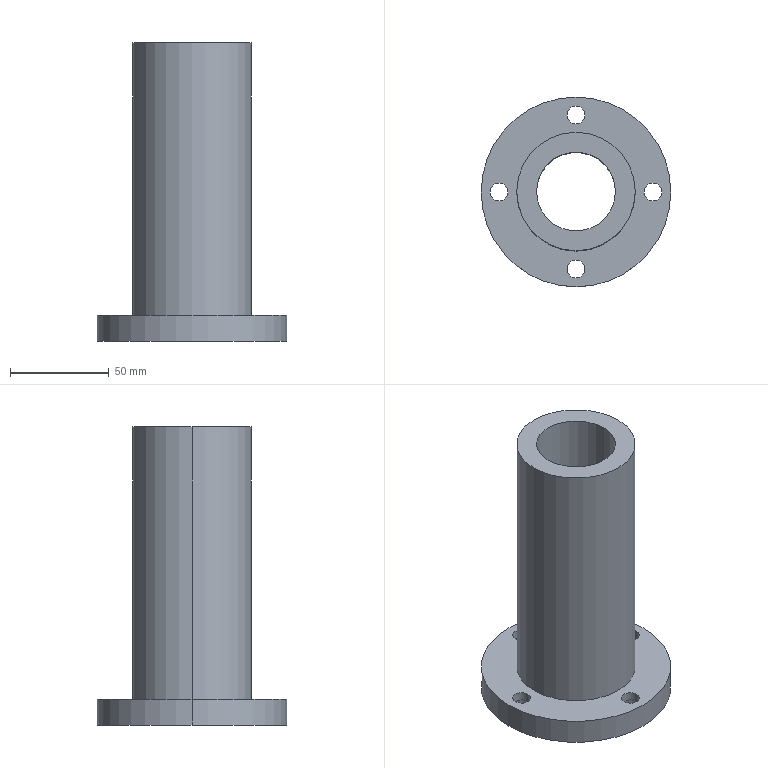Part | SolidWorks | features ICE 2, 3DProfileFeature 1, Extrusion 1, HoleWzd 1 | 1 solid | 29 faces | box 96 x 96 x 151 mm | volume 288115 mm3 | cylinder 22 | plane 7 | commonest cylinder face diameters 9 x8 14 x8 40 x2 60 x2 96 x2
STEP:
#1=CARTESIAN_POINT('',(-20.,0.,0.));
#2=VERTEX_POINT('',#1);
#3=CARTESIAN_POINT('',(20.,0.,0.));
#4=VERTEX_POINT('',#3);
#5=CARTESIAN_POINT('',(0.,0.,0.));
#6=DIRECTION('',(0.,0.,1.));
#7=DIRECTION('',(1.,0.,0.));
#8=AXIS2_PLACEMENT_3D('',#5,#6,#7);
#9=CIRCLE('',#8,20.);
#10=EDGE_CURVE('',#2,#4,#9,.T.);
#11=ORIENTED_EDGE('',*,*,#10,.F.);
#12=CARTESIAN_POINT('',(-20.,0.,151.));
#13=VERTEX_POINT('',#12);
#14=CARTESIAN_POINT('',(-20.,0.,0.));
#15=DIRECTION('',(0.,0.,1.));
#16=VECTOR('',#15,1000.);
#17=LINE('',#14,#16);
#18=EDGE_CURVE('',#2,#13,#17,.T.);
#19=ORIENTED_EDGE('',*,*,#18,.T.);
#20=CARTESIAN_POINT('',(20.,0.,151.));
#21=VERTEX_POINT('',#20);
#22=CARTESIAN_POINT('',(0.,0.,151.));
#23=DIRECTION('',(0.,0.,1.));
#24=DIRECTION('',(1.,0.,0.));
#25=AXIS2_PLACEMENT_3D('',#22,#23,#24);
#26=CIRCLE('',#25,20.);
#27=EDGE_CURVE('',#13,#21,#26,.T.);
#28=ORIENTED_EDGE('',*,*,#27,.T.);
#29=CARTESIAN_POINT('',(20.,0.,0.));
#30=DIRECTION('',(0.,0.,1.));
#31=VECTOR('',#30,1000.);
#32=LINE('',#29,#31);
#33=EDGE_CURVE('',#4,#21,#32,.T.);
#34=ORIENTED_EDGE('',*,*,#33,.F.);
#35=EDGE_LOOP('',(#11,#19,#28,#34));
#36=FACE_OUTER_BOUND('',#35,.T.);
#37=CARTESIAN_POINT('',(0.,0.,0.));
#38=DIRECTION('',(0.,0.,1.));
#39=DIRECTION('',(1.,0.,0.));
#40=AXIS2_PLACEMENT_3D('',#37,#38,#39);
#41=CYLINDRICAL_SURFACE('',#40,20.);
#42=ADVANCED_FACE('',(#36),#41,.F.);
#43=CARTESIAN_POINT('',(30.,0.,151.));
#44=VERTEX_POINT('',#43);
#45=CARTESIAN_POINT('',(-30.,0.,151.));
#46=VERTEX_POINT('',#45);
#47=CARTESIAN_POINT('',(0.,0.,151.));
#48=DIRECTION('',(0.,0.,1.));
#49=DIRECTION('',(1.,0.,0.));
#50=AXIS2_PLACEMENT_3D('',#47,#48,#49);
#51=CIRCLE('',#50,30.);
#52=EDGE_CURVE('',#44,#46,#51,.T.);
#53=ORIENTED_EDGE('',*,*,#52,.F.);
#54=CARTESIAN_POINT('',(30.,0.,13.));
#55=VERTEX_POINT('',#54);
#56=CARTESIAN_POINT('',(30.,0.,151.));
#57=DIRECTION('',(0.,0.,-1.));
#58=VECTOR('',#57,1000.);
#59=LINE('',#56,#58);
#60=EDGE_CURVE('',#44,#55,#59,.T.);
#61=ORIENTED_EDGE('',*,*,#60,.T.);
#62=CARTESIAN_POINT('',(-30.,0.,13.));
#63=VERTEX_POINT('',#62);
#64=CARTESIAN_POINT('',(0.,0.,13.));
#65=DIRECTION('',(0.,0.,1.));
#66=DIRECTION('',(1.,0.,0.));
#67=AXIS2_PLACEMENT_3D('',#64,#65,#66);
#68=CIRCLE('',#67,30.);
#69=EDGE_CURVE('',#55,#63,#68,.T.);
#70=ORIENTED_EDGE('',*,*,#69,.T.);
#71=CARTESIAN_POINT('',(-30.,0.,151.));
#72=DIRECTION('',(0.,0.,-1.));
#73=VECTOR('',#72,1000.);
#74=LINE('',#71,#73);
#75=EDGE_CURVE('',#46,#63,#74,.T.);
#76=ORIENTED_EDGE('',*,*,#75,.F.);
#77=EDGE_LOOP('',(#53,#61,#70,#76));
#78=FACE_OUTER_BOUND('',#77,.T.);
#79=CARTESIAN_POINT('',(0.,0.,151.));
#80=DIRECTION('',(0.,0.,-1.));
#81=DIRECTION('',(-1.,0.,0.));
#82=AXIS2_PLACEMENT_3D('',#79,#80,#81);
#83=CYLINDRICAL_SURFACE('',#82,30.);
#84=ADVANCED_FACE('',(#78),#83,.T.);
#85=CARTESIAN_POINT('',(7.,39.,8.6));
#86=VERTEX_POINT('',#85);
#87=CARTESIAN_POINT('',(-7.,39.,8.6));
#88=VERTEX_POINT('',#87);
#89=CARTESIAN_POINT('',(0.,39.,8.6));
#90=DIRECTION('',(0.,0.,-1.));
#91=DIRECTION('',(-1.,0.,0.));
#92=AXIS2_PLACEMENT_3D('',#89,#90,#91);
#93=CIRCLE('',#92,7.);
#94=EDGE_CURVE('',#86,#88,#93,.T.);
#95=ORIENTED_EDGE('',*,*,#94,.F.);
#96=CARTESIAN_POINT('',(7.,39.,0.));
#97=VERTEX_POINT('',#96);
#98=CARTESIAN_POINT('',(7.,39.,0.));
#99=DIRECTION('',(0.,0.,-1.));
#100=VECTOR('',#99,1000.);
#101=LINE('',#98,#100);
#102=EDGE_CURVE('',#86,#97,#101,.T.);
#103=ORIENTED_EDGE('',*,*,#102,.T.);
#104=CARTESIAN_POINT('',(-7.,39.,0.));
#105=VERTEX_POINT('',#104);
#106=CARTESIAN_POINT('',(0.,39.,0.));
#107=DIRECTION('',(0.,0.,-1.));
#108=DIRECTION('',(-1.,0.,0.));
#109=AXIS2_PLACEMENT_3D('',#106,#107,#108);
#110=CIRCLE('',#109,7.);
#111=EDGE_CURVE('',#97,#105,#110,.T.);
#112=ORIENTED_EDGE('',*,*,#111,.T.);
#113=CARTESIAN_POINT('',(-7.,39.,0.));
#114=DIRECTION('',(0.,0.,-1.));
#115=VECTOR('',#114,1000.);
#116=LINE('',#113,#115);
#117=EDGE_CURVE('',#88,#105,#116,.T.);
#118=ORIENTED_EDGE('',*,*,#117,.F.);
#119=EDGE_LOOP('',(#95,#103,#112,#118));
#120=FACE_OUTER_BOUND('',#119,.T.);
#121=CARTESIAN_POINT('',(0.,39.,0.));
#122=DIRECTION('',(0.,0.,-1.));
#123=DIRECTION('',(-1.,0.,0.));
#124=AXIS2_PLACEMENT_3D('',#121,#122,#123);
#125=CYLINDRICAL_SURFACE('',#124,7.);
#126=ADVANCED_FACE('',(#120),#125,.F.);
#127=CARTESIAN_POINT('',(4.5,39.,13.));
#128=VERTEX_POINT('',#127);
#129=CARTESIAN_POINT('',(-4.5,39.,13.));
#130=VERTEX_POINT('',#129);
#131=CARTESIAN_POINT('',(0.,39.,13.));
#132=DIRECTION('',(0.,0.,-1.));
#133=DIRECTION('',(-1.,0.,0.));
#134=AXIS2_PLACEMENT_3D('',#131,#132,#133);
#135=CIRCLE('',#134,4.5);
#136=EDGE_CURVE('',#128,#130,#135,.T.);
#137=ORIENTED_EDGE('',*,*,#136,.F.);
#138=CARTESIAN_POINT('',(4.5,39.,8.6));
#139=VERTEX_POINT('',#138);
#140=CARTESIAN_POINT('',(4.5,39.,0.));
#141=DIRECTION('',(0.,0.,-1.));
#142=VECTOR('',#141,1000.);
#143=LINE('',#140,#142);
#144=EDGE_CURVE('',#128,#139,#143,.T.);
#145=ORIENTED_EDGE('',*,*,#144,.T.);
#146=CARTESIAN_POINT('',(-4.5,39.,8.6));
#147=VERTEX_POINT('',#146);
#148=CARTESIAN_POINT('',(0.,39.,8.6));
#149=DIRECTION('',(0.,0.,-1.));
#150=DIRECTION('',(-1.,0.,0.));
#151=AXIS2_PLACEMENT_3D('',#148,#149,#150);
#152=CIRCLE('',#151,4.5);
#153=EDGE_CURVE('',#139,#147,#152,.T.);
#154=ORIENTED_EDGE('',*,*,#153,.T.);
#155=CARTESIAN_POINT('',(-4.5,39.,0.));
#156=DIRECTION('',(0.,0.,-1.));
#157=VECTOR('',#156,1000.);
#158=LINE('',#155,#157);
#159=EDGE_CURVE('',#130,#147,#158,.T.);
#160=ORIENTED_EDGE('',*,*,#159,.F.);
#161=EDGE_LOOP('',(#137,#145,#154,#160));
#162=FACE_OUTER_BOUND('',#161,.T.);
#163=CARTESIAN_POINT('',(0.,39.,0.));
#164=DIRECTION('',(0.,0.,-1.));
#165=DIRECTION('',(-1.,0.,0.));
#166=AXIS2_PLACEMENT_3D('',#163,#164,#165);
#167=CYLINDRICAL_SURFACE('',#166,4.5);
#168=ADVANCED_FACE('',(#162),#167,.F.);
#169=CARTESIAN_POINT('',(46.,0.,8.6));
#170=VERTEX_POINT('',#169);
#171=CARTESIAN_POINT('',(32.,0.,8.6));
#172=VERTEX_POINT('',#171);
#173=CARTESIAN_POINT('',(39.,0.,8.6));
#174=DIRECTION('',(0.,0.,-1.));
#175=DIRECTION('',(-1.,0.,0.));
#176=AXIS2_PLACEMENT_3D('',#173,#174,#175);
#177=CIRCLE('',#176,7.);
#178=EDGE_CURVE('',#170,#172,#177,.T.);
#179=ORIENTED_EDGE('',*,*,#178,.F.);
#180=CARTESIAN_POINT('',(46.,0.,0.));
#181=VERTEX_POINT('',#180);
#182=CARTESIAN_POINT('',(46.,0.,0.));
#183=DIRECTION('',(0.,0.,-1.));
#184=VECTOR('',#183,1000.);
#185=LINE('',#182,#184);
#186=EDGE_CURVE('',#170,#181,#185,.T.);
#187=ORIENTED_EDGE('',*,*,#186,.T.);
#188=CARTESIAN_POINT('',(32.,0.,0.));
#189=VERTEX_POINT('',#188);
#190=CARTESIAN_POINT('',(39.,0.,0.));
#191=DIRECTION('',(0.,0.,-1.));
#192=DIRECTION('',(-1.,0.,0.));
#193=AXIS2_PLACEMENT_3D('',#190,#191,#192);
#194=CIRCLE('',#193,7.);
#195=EDGE_CURVE('',#181,#189,#194,.T.);
#196=ORIENTED_EDGE('',*,*,#195,.T.);
#197=CARTESIAN_POINT('',(32.,0.,0.));
#198=DIRECTION('',(0.,0.,-1.));
#199=VECTOR('',#198,1000.);
#200=LINE('',#197,#199);
#201=EDGE_CURVE('',#172,#189,#200,.T.);
#202=ORIENTED_EDGE('',*,*,#201,.F.);
#203=EDGE_LOOP('',(#179,#187,#196,#202));
#204=FACE_OUTER_BOUND('',#203,.T.);
#205=CARTESIAN_POINT('',(39.,0.,0.));
#206=DIRECTION('',(0.,0.,-1.));
#207=DIRECTION('',(-1.,0.,0.));
#208=AXIS2_PLACEMENT_3D('',#205,#206,#207);
#209=CYLINDRICAL_SURFACE('',#208,7.);
#210=ADVANCED_FACE('',(#204),#209,.F.);
#211=CARTESIAN_POINT('',(43.5,0.,13.));
#212=VERTEX_POINT('',#211);
#213=CARTESIAN_POINT('',(34.5,0.,13.));
#214=VERTEX_POINT('',#213);
#215=CARTESIAN_POINT('',(39.,0.,13.));
#216=DIRECTION('',(0.,0.,-1.));
#217=DIRECTION('',(-1.,0.,0.));
#218=AXIS2_PLACEMENT_3D('',#215,#216,#217);
#219=CIRCLE('',#218,4.5);
#220=EDGE_CURVE('',#212,#214,#219,.T.);
#221=ORIENTED_EDGE('',*,*,#220,.F.);
#222=CARTESIAN_POINT('',(43.5,0.,8.6));
#223=VERTEX_POINT('',#222);
#224=CARTESIAN_POINT('',(43.5,0.,0.));
#225=DIRECTION('',(0.,0.,-1.));
#226=VECTOR('',#225,1000.);
#227=LINE('',#224,#226);
#228=EDGE_CURVE('',#212,#223,#227,.T.);
#229=ORIENTED_EDGE('',*,*,#228,.T.);
#230=CARTESIAN_POINT('',(34.5,0.,8.6));
#231=VERTEX_POINT('',#230);
#232=CARTESIAN_POINT('',(39.,0.,8.6));
#233=DIRECTION('',(0.,0.,-1.));
#234=DIRECTION('',(-1.,0.,0.));
#235=AXIS2_PLACEMENT_3D('',#232,#233,#234);
#236=CIRCLE('',#235,4.5);
#237=EDGE_CURVE('',#223,#231,#236,.T.);
#238=ORIENTED_EDGE('',*,*,#237,.T.);
#239=CARTESIAN_POINT('',(34.5,0.,0.));
#240=DIRECTION('',(0.,0.,-1.));
#241=VECTOR('',#240,1000.);
#242=LINE('',#239,#241);
#243=EDGE_CURVE('',#214,#231,#242,.T.);
#244=ORIENTED_EDGE('',*,*,#243,.F.);
#245=EDGE_LOOP('',(#221,#229,#238,#244));
#246=FACE_OUTER_BOUND('',#245,.T.);
#247=CARTESIAN_POINT('',(39.,0.,0.));
#248=DIRECTION('',(0.,0.,-1.));
#249=DIRECTION('',(-1.,0.,0.));
#250=AXIS2_PLACEMENT_3D('',#247,#248,#249);
#251=CYLINDRICAL_SURFACE('',#250,4.5);
#252=ADVANCED_FACE('',(#246),#251,.F.);
#253=CARTESIAN_POINT('',(7.,-39.,8.6));
#254=VERTEX_POINT('',#253);
#255=CARTESIAN_POINT('',(-7.,-39.,8.6));
#256=VERTEX_POINT('',#255);
#257=CARTESIAN_POINT('',(0.,-39.,8.6));
#258=DIRECTION('',(0.,0.,-1.));
#259=DIRECTION('',(-1.,0.,0.));
#260=AXIS2_PLACEMENT_3D('',#257,#258,#259);
#261=CIRCLE('',#260,7.);
#262=EDGE_CURVE('',#254,#256,#261,.T.);
#263=ORIENTED_EDGE('',*,*,#262,.F.);
#264=CARTESIAN_POINT('',(7.,-39.,0.));
#265=VERTEX_POINT('',#264);
#266=CARTESIAN_POINT('',(7.,-39.,0.));
#267=DIRECTION('',(0.,0.,-1.));
#268=VECTOR('',#267,1000.);
#269=LINE('',#266,#268);
#270=EDGE_CURVE('',#254,#265,#269,.T.);
#271=ORIENTED_EDGE('',*,*,#270,.T.);
#272=CARTESIAN_POINT('',(-7.,-39.,0.));
#273=VERTEX_POINT('',#272);
#274=CARTESIAN_POINT('',(0.,-39.,0.));
#275=DIRECTION('',(0.,0.,-1.));
#276=DIRECTION('',(-1.,0.,0.));
#277=AXIS2_PLACEMENT_3D('',#274,#275,#276);
#278=CIRCLE('',#277,7.);
#279=EDGE_CURVE('',#265,#273,#278,.T.);
#280=ORIENTED_EDGE('',*,*,#279,.T.);
#281=CARTESIAN_POINT('',(-7.,-39.,0.));
#282=DIRECTION('',(0.,0.,-1.));
#283=VECTOR('',#282,1000.);
#284=LINE('',#281,#283);
#285=EDGE_CURVE('',#256,#273,#284,.T.);
#286=ORIENTED_EDGE('',*,*,#285,.F.);
#287=EDGE_LOOP('',(#263,#271,#280,#286));
#288=FACE_OUTER_BOUND('',#287,.T.);
#289=CARTESIAN_POINT('',(0.,-39.,0.));
#290=DIRECTION('',(0.,0.,-1.));
#291=DIRECTION('',(-1.,0.,0.));
#292=AXIS2_PLACEMENT_3D('',#289,#290,#291);
#293=CYLINDRICAL_SURFACE('',#292,7.);
#294=ADVANCED_FACE('',(#288),#293,.F.);
#295=CARTESIAN_POINT('',(4.5,-39.,13.));
#296=VERTEX_POINT('',#295);
#297=CARTESIAN_POINT('',(-4.5,-39.,13.));
#298=VERTEX_POINT('',#297);
#299=CARTESIAN_POINT('',(0.,-39.,13.));
#300=DIRECTION('',(0.,0.,-1.));
#301=DIRECTION('',(-1.,0.,0.));
#302=AXIS2_PLACEMENT_3D('',#299,#300,#301);
#303=CIRCLE('',#302,4.5);
#304=EDGE_CURVE('',#296,#298,#303,.T.);
#305=ORIENTED_EDGE('',*,*,#304,.F.);
#306=CARTESIAN_POINT('',(4.5,-39.,8.6));
#307=VERTEX_POINT('',#306);
#308=CARTESIAN_POINT('',(4.5,-39.,0.));
#309=DIRECTION('',(0.,0.,-1.));
#310=VECTOR('',#309,1000.);
#311=LINE('',#308,#310);
#312=EDGE_CURVE('',#296,#307,#311,.T.);
#313=ORIENTED_EDGE('',*,*,#312,.T.);
#314=CARTESIAN_POINT('',(-4.5,-39.,8.6));
#315=VERTEX_POINT('',#314);
#316=CARTESIAN_POINT('',(0.,-39.,8.6));
#317=DIRECTION('',(0.,0.,-1.));
#318=DIRECTION('',(-1.,0.,0.));
#319=AXIS2_PLACEMENT_3D('',#316,#317,#318);
#320=CIRCLE('',#319,4.5);
#321=EDGE_CURVE('',#307,#315,#320,.T.);
#322=ORIENTED_EDGE('',*,*,#321,.T.);
#323=CARTESIAN_POINT('',(-4.5,-39.,0.));
#324=DIRECTION('',(0.,0.,-1.));
#325=VECTOR('',#324,1000.);
#326=LINE('',#323,#325);
#327=EDGE_CURVE('',#298,#315,#326,.T.);
#328=ORIENTED_EDGE('',*,*,#327,.F.);
#329=EDGE_LOOP('',(#305,#313,#322,#328));
#330=FACE_OUTER_BOUND('',#329,.T.);
#331=CARTESIAN_POINT('',(0.,-39.,0.));
#332=DIRECTION('',(0.,0.,-1.));
#333=DIRECTION('',(-1.,0.,0.));
#334=AXIS2_PLACEMENT_3D('',#331,#332,#333);
#335=CYLINDRICAL_SURFACE('',#334,4.5);
#336=ADVANCED_FACE('',(#330),#335,.F.);
#337=CARTESIAN_POINT('',(-32.,0.,8.6));
#338=VERTEX_POINT('',#337);
#339=CARTESIAN_POINT('',(-46.,0.,8.6));
#340=VERTEX_POINT('',#339);
#341=CARTESIAN_POINT('',(-39.,0.,8.6));
#342=DIRECTION('',(0.,0.,-1.));
#343=DIRECTION('',(-1.,0.,0.));
#344=AXIS2_PLACEMENT_3D('',#341,#342,#343);
#345=CIRCLE('',#344,7.);
#346=EDGE_CURVE('',#338,#340,#345,.T.);
#347=ORIENTED_EDGE('',*,*,#346,.F.);
#348=CARTESIAN_POINT('',(-32.,0.,0.));
#349=VERTEX_POINT('',#348);
#350=CARTESIAN_POINT('',(-32.,0.,0.));
#351=DIRECTION('',(0.,0.,-1.));
#352=VECTOR('',#351,1000.);
#353=LINE('',#350,#352);
#354=EDGE_CURVE('',#338,#349,#353,.T.);
#355=ORIENTED_EDGE('',*,*,#354,.T.);
#356=CARTESIAN_POINT('',(-46.,0.,0.));
#357=VERTEX_POINT('',#356);
#358=CARTESIAN_POINT('',(-39.,0.,0.));
#359=DIRECTION('',(0.,0.,-1.));
#360=DIRECTION('',(-1.,0.,0.));
#361=AXIS2_PLACEMENT_3D('',#358,#359,#360);
#362=CIRCLE('',#361,7.);
#363=EDGE_CURVE('',#349,#357,#362,.T.);
#364=ORIENTED_EDGE('',*,*,#363,.T.);
#365=CARTESIAN_POINT('',(-46.,0.,0.));
#366=DIRECTION('',(0.,0.,-1.));
#367=VECTOR('',#366,1000.);
#368=LINE('',#365,#367);
#369=EDGE_CURVE('',#340,#357,#368,.T.);
#370=ORIENTED_EDGE('',*,*,#369,.F.);
#371=EDGE_LOOP('',(#347,#355,#364,#370));
#372=FACE_OUTER_BOUND('',#371,.T.);
#373=CARTESIAN_POINT('',(-39.,0.,0.));
#374=DIRECTION('',(0.,0.,-1.));
#375=DIRECTION('',(-1.,0.,0.));
#376=AXIS2_PLACEMENT_3D('',#373,#374,#375);
#377=CYLINDRICAL_SURFACE('',#376,7.);
#378=ADVANCED_FACE('',(#372),#377,.F.);
#379=CARTESIAN_POINT('',(-34.5,0.,13.));
#380=VERTEX_POINT('',#379);
#381=CARTESIAN_POINT('',(-43.5,0.,13.));
#382=VERTEX_POINT('',#381);
#383=CARTESIAN_POINT('',(-39.,0.,13.));
#384=DIRECTION('',(0.,0.,-1.));
#385=DIRECTION('',(-1.,0.,0.));
#386=AXIS2_PLACEMENT_3D('',#383,#384,#385);
#387=CIRCLE('',#386,4.5);
#388=EDGE_CURVE('',#380,#382,#387,.T.);
#389=ORIENTED_EDGE('',*,*,#388,.F.);
#390=CARTESIAN_POINT('',(-34.5,0.,8.6));
#391=VERTEX_POINT('',#390);
#392=CARTESIAN_POINT('',(-34.5,0.,0.));
#393=DIRECTION('',(0.,0.,-1.));
#394=VECTOR('',#393,1000.);
#395=LINE('',#392,#394);
#396=EDGE_CURVE('',#380,#391,#395,.T.);
#397=ORIENTED_EDGE('',*,*,#396,.T.);
#398=CARTESIAN_POINT('',(-43.5,0.,8.6));
#399=VERTEX_POINT('',#398);
#400=CARTESIAN_POINT('',(-39.,0.,8.6));
#401=DIRECTION('',(0.,0.,-1.));
#402=DIRECTION('',(-1.,0.,0.));
#403=AXIS2_PLACEMENT_3D('',#400,#401,#402);
#404=CIRCLE('',#403,4.5);
#405=EDGE_CURVE('',#391,#399,#404,.T.);
#406=ORIENTED_EDGE('',*,*,#405,.T.);
#407=CARTESIAN_POINT('',(-43.5,0.,0.));
#408=DIRECTION('',(0.,0.,-1.));
#409=VECTOR('',#408,1000.);
#410=LINE('',#407,#409);
#411=EDGE_CURVE('',#382,#399,#410,.T.);
#412=ORIENTED_EDGE('',*,*,#411,.F.);
#413=EDGE_LOOP('',(#389,#397,#406,#412));
#414=FACE_OUTER_BOUND('',#413,.T.);
#415=CARTESIAN_POINT('',(-39.,0.,0.));
#416=DIRECTION('',(0.,0.,-1.));
#417=DIRECTION('',(-1.,0.,0.));
#418=AXIS2_PLACEMENT_3D('',#415,#416,#417);
#419=CYLINDRICAL_SURFACE('',#418,4.5);
#420=ADVANCED_FACE('',(#414),#419,.F.);
#421=CARTESIAN_POINT('',(48.,0.,13.));
#422=VERTEX_POINT('',#421);
#423=CARTESIAN_POINT('',(-48.,0.,13.));
#424=VERTEX_POINT('',#423);
#425=CARTESIAN_POINT('',(0.,0.,13.));
#426=DIRECTION('',(0.,0.,1.));
#427=DIRECTION('',(1.,0.,0.));
#428=AXIS2_PLACEMENT_3D('',#425,#426,#427);
#429=CIRCLE('',#428,48.);
#430=EDGE_CURVE('',#422,#424,#429,.T.);
#431=ORIENTED_EDGE('',*,*,#430,.F.);
#432=CARTESIAN_POINT('',(48.,0.,0.));
#433=VERTEX_POINT('',#432);
#434=CARTESIAN_POINT('',(48.,0.,13.));
#435=DIRECTION('',(0.,0.,-1.));
#436=VECTOR('',#435,1000.);
#437=LINE('',#434,#436);
#438=EDGE_CURVE('',#422,#433,#437,.T.);
#439=ORIENTED_EDGE('',*,*,#438,.T.);
#440=CARTESIAN_POINT('',(-48.,0.,0.));
#441=VERTEX_POINT('',#440);
#442=CARTESIAN_POINT('',(0.,0.,0.));
#443=DIRECTION('',(0.,0.,1.));
#444=DIRECTION('',(1.,0.,0.));
#445=AXIS2_PLACEMENT_3D('',#442,#443,#444);
#446=CIRCLE('',#445,48.);
#447=EDGE_CURVE('',#433,#441,#446,.T.);
#448=ORIENTED_EDGE('',*,*,#447,.T.);
#449=CARTESIAN_POINT('',(-48.,0.,13.));
#450=DIRECTION('',(0.,0.,-1.));
#451=VECTOR('',#450,1000.);
#452=LINE('',#449,#451);
#453=EDGE_CURVE('',#424,#441,#452,.T.);
#454=ORIENTED_EDGE('',*,*,#453,.F.);
#455=EDGE_LOOP('',(#431,#439,#448,#454));
#456=FACE_OUTER_BOUND('',#455,.T.);
#457=CARTESIAN_POINT('',(0.,0.,13.));
#458=DIRECTION('',(0.,0.,-1.));
#459=DIRECTION('',(-1.,0.,0.));
#460=AXIS2_PLACEMENT_3D('',#457,#458,#459);
#461=CYLINDRICAL_SURFACE('',#460,48.);
#462=ADVANCED_FACE('',(#456),#461,.T.);
#463=CARTESIAN_POINT('',(0.,0.,13.));
#464=DIRECTION('',(0.,0.,1.));
#465=DIRECTION('',(1.,0.,0.));
#466=AXIS2_PLACEMENT_3D('',#463,#464,#465);
#467=CIRCLE('',#466,48.);
#468=EDGE_CURVE('',#424,#422,#467,.T.);
#469=ORIENTED_EDGE('',*,*,#468,.T.);
#470=ORIENTED_EDGE('',*,*,#430,.T.);
#471=EDGE_LOOP('',(#469,#470));
#472=FACE_OUTER_BOUND('',#471,.T.);
#473=CARTESIAN_POINT('',(-39.,0.,13.));
#474=DIRECTION('',(0.,0.,-1.));
#475=DIRECTION('',(-1.,0.,0.));
#476=AXIS2_PLACEMENT_3D('',#473,#474,#475);
#477=CIRCLE('',#476,4.5);
#478=EDGE_CURVE('',#382,#380,#477,.T.);
#479=ORIENTED_EDGE('',*,*,#478,.T.);
#480=ORIENTED_EDGE('',*,*,#388,.T.);
#481=EDGE_LOOP('',(#479,#480));
#482=FACE_BOUND('',#481,.T.);
#483=CARTESIAN_POINT('',(0.,-39.,13.));
#484=DIRECTION('',(0.,0.,-1.));
#485=DIRECTION('',(-1.,0.,0.));
#486=AXIS2_PLACEMENT_3D('',#483,#484,#485);
#487=CIRCLE('',#486,4.5);
#488=EDGE_CURVE('',#298,#296,#487,.T.);
#489=ORIENTED_EDGE('',*,*,#488,.T.);
#490=ORIENTED_EDGE('',*,*,#304,.T.);
#491=EDGE_LOOP('',(#489,#490));
#492=FACE_BOUND('',#491,.T.);
#493=CARTESIAN_POINT('',(39.,0.,13.));
#494=DIRECTION('',(0.,0.,-1.));
#495=DIRECTION('',(-1.,0.,0.));
#496=AXIS2_PLACEMENT_3D('',#493,#494,#495);
#497=CIRCLE('',#496,4.5);
#498=EDGE_CURVE('',#214,#212,#497,.T.);
#499=ORIENTED_EDGE('',*,*,#498,.T.);
#500=ORIENTED_EDGE('',*,*,#220,.T.);
#501=EDGE_LOOP('',(#499,#500));
#502=FACE_BOUND('',#501,.T.);
#503=CARTESIAN_POINT('',(0.,39.,13.));
#504=DIRECTION('',(0.,0.,-1.));
#505=DIRECTION('',(-1.,0.,0.));
#506=AXIS2_PLACEMENT_3D('',#503,#504,#505);
#507=CIRCLE('',#506,4.5);
#508=EDGE_CURVE('',#130,#128,#507,.T.);
#509=ORIENTED_EDGE('',*,*,#508,.T.);
#510=ORIENTED_EDGE('',*,*,#136,.T.);
#511=EDGE_LOOP('',(#509,#510));
#512=FACE_BOUND('',#511,.T.);
#513=CARTESIAN_POINT('',(0.,0.,13.));
#514=DIRECTION('',(0.,0.,1.));
#515=DIRECTION('',(1.,0.,0.));
#516=AXIS2_PLACEMENT_3D('',#513,#514,#515);
#517=CIRCLE('',#516,30.);
#518=EDGE_CURVE('',#63,#55,#517,.T.);
#519=ORIENTED_EDGE('',*,*,#518,.F.);
#520=ORIENTED_EDGE('',*,*,#69,.F.);
#521=EDGE_LOOP('',(#519,#520));
#522=FACE_BOUND('',#521,.T.);
#523=CARTESIAN_POINT('',(0.,0.,13.));
#524=DIRECTION('',(0.,0.,1.));
#525=DIRECTION('',(1.,0.,0.));
#526=AXIS2_PLACEMENT_3D('',#523,#524,#525);
#527=PLANE('',#526);
#528=ADVANCED_FACE('',(#472,#482,#492,#502,#512,#522),#527,.T.);
#529=ORIENTED_EDGE('',*,*,#438,.F.);
#530=ORIENTED_EDGE('',*,*,#468,.F.);
#531=ORIENTED_EDGE('',*,*,#453,.T.);
#532=CARTESIAN_POINT('',(0.,0.,0.));
#533=DIRECTION('',(0.,0.,1.));
#534=DIRECTION('',(1.,0.,0.));
#535=AXIS2_PLACEMENT_3D('',#532,#533,#534);
#536=CIRCLE('',#535,48.);
#537=EDGE_CURVE('',#441,#433,#536,.T.);
#538=ORIENTED_EDGE('',*,*,#537,.T.);
#539=EDGE_LOOP('',(#529,#530,#531,#538));
#540=FACE_OUTER_BOUND('',#539,.T.);
#541=CARTESIAN_POINT('',(0.,0.,13.));
#542=DIRECTION('',(0.,0.,-1.));
#543=DIRECTION('',(-1.,0.,0.));
#544=AXIS2_PLACEMENT_3D('',#541,#542,#543);
#545=CYLINDRICAL_SURFACE('',#544,48.);
#546=ADVANCED_FACE('',(#540),#545,.T.);
#547=CARTESIAN_POINT('',(0.,0.,0.));
#548=DIRECTION('',(0.,0.,1.));
#549=DIRECTION('',(1.,0.,0.));
#550=AXIS2_PLACEMENT_3D('',#547,#548,#549);
#551=CIRCLE('',#550,20.);
#552=EDGE_CURVE('',#4,#2,#551,.T.);
#553=ORIENTED_EDGE('',*,*,#552,.T.);
#554=ORIENTED_EDGE('',*,*,#10,.T.);
#555=EDGE_LOOP('',(#553,#554));
#556=FACE_BOUND('',#555,.T.);
#557=CARTESIAN_POINT('',(0.,39.,0.));
#558=DIRECTION('',(0.,0.,-1.));
#559=DIRECTION('',(-1.,0.,0.));
#560=AXIS2_PLACEMENT_3D('',#557,#558,#559);
#561=CIRCLE('',#560,7.);
#562=EDGE_CURVE('',#105,#97,#561,.T.);
#563=ORIENTED_EDGE('',*,*,#562,.F.);
#564=ORIENTED_EDGE('',*,*,#111,.F.);
#565=EDGE_LOOP('',(#563,#564));
#566=FACE_BOUND('',#565,.T.);
#567=CARTESIAN_POINT('',(39.,0.,0.));
#568=DIRECTION('',(0.,0.,-1.));
#569=DIRECTION('',(-1.,0.,0.));
#570=AXIS2_PLACEMENT_3D('',#567,#568,#569);
#571=CIRCLE('',#570,7.);
#572=EDGE_CURVE('',#189,#181,#571,.T.);
#573=ORIENTED_EDGE('',*,*,#572,.F.);
#574=ORIENTED_EDGE('',*,*,#195,.F.);
#575=EDGE_LOOP('',(#573,#574));
#576=FACE_BOUND('',#575,.T.);
#577=CARTESIAN_POINT('',(0.,-39.,0.));
#578=DIRECTION('',(0.,0.,-1.));
#579=DIRECTION('',(-1.,0.,0.));
#580=AXIS2_PLACEMENT_3D('',#577,#578,#579);
#581=CIRCLE('',#580,7.);
#582=EDGE_CURVE('',#273,#265,#581,.T.);
#583=ORIENTED_EDGE('',*,*,#582,.F.);
#584=ORIENTED_EDGE('',*,*,#279,.F.);
#585=EDGE_LOOP('',(#583,#584));
#586=FACE_BOUND('',#585,.T.);
#587=CARTESIAN_POINT('',(-39.,0.,0.));
#588=DIRECTION('',(0.,0.,-1.));
#589=DIRECTION('',(-1.,0.,0.));
#590=AXIS2_PLACEMENT_3D('',#587,#588,#589);
#591=CIRCLE('',#590,7.);
#592=EDGE_CURVE('',#357,#349,#591,.T.);
#593=ORIENTED_EDGE('',*,*,#592,.F.);
#594=ORIENTED_EDGE('',*,*,#363,.F.);
#595=EDGE_LOOP('',(#593,#594));
#596=FACE_BOUND('',#595,.T.);
#597=ORIENTED_EDGE('',*,*,#537,.F.);
#598=ORIENTED_EDGE('',*,*,#447,.F.);
#599=EDGE_LOOP('',(#597,#598));
#600=FACE_OUTER_BOUND('',#599,.T.);
#601=CARTESIAN_POINT('',(0.,0.,0.));
#602=DIRECTION('',(0.,0.,1.));
#603=DIRECTION('',(1.,0.,0.));
#604=AXIS2_PLACEMENT_3D('',#601,#602,#603);
#605=PLANE('',#604);
#606=ADVANCED_FACE('',(#556,#566,#576,#586,#596,#600),#605,.F.);
#607=ORIENTED_EDGE('',*,*,#396,.F.);
#608=ORIENTED_EDGE('',*,*,#478,.F.);
#609=ORIENTED_EDGE('',*,*,#411,.T.);
#610=CARTESIAN_POINT('',(-39.,0.,8.6));
#611=DIRECTION('',(0.,0.,-1.));
#612=DIRECTION('',(-1.,0.,0.));
#613=AXIS2_PLACEMENT_3D('',#610,#611,#612);
#614=CIRCLE('',#613,4.5);
#615=EDGE_CURVE('',#399,#391,#614,.T.);
#616=ORIENTED_EDGE('',*,*,#615,.T.);
#617=EDGE_LOOP('',(#607,#608,#609,#616));
#618=FACE_OUTER_BOUND('',#617,.T.);
#619=CARTESIAN_POINT('',(-39.,0.,0.));
#620=DIRECTION('',(0.,0.,-1.));
#621=DIRECTION('',(-1.,0.,0.));
#622=AXIS2_PLACEMENT_3D('',#619,#620,#621);
#623=CYLINDRICAL_SURFACE('',#622,4.5);
#624=ADVANCED_FACE('',(#618),#623,.F.);
#625=ORIENTED_EDGE('',*,*,#615,.F.);
#626=ORIENTED_EDGE('',*,*,#405,.F.);
#627=EDGE_LOOP('',(#625,#626));
#628=FACE_BOUND('',#627,.T.);
#629=CARTESIAN_POINT('',(-39.,0.,8.6));
#630=DIRECTION('',(0.,0.,-1.));
#631=DIRECTION('',(-1.,0.,0.));
#632=AXIS2_PLACEMENT_3D('',#629,#630,#631);
#633=CIRCLE('',#632,7.);
#634=EDGE_CURVE('',#340,#338,#633,.T.);
#635=ORIENTED_EDGE('',*,*,#634,.T.);
#636=ORIENTED_EDGE('',*,*,#346,.T.);
#637=EDGE_LOOP('',(#635,#636));
#638=FACE_OUTER_BOUND('',#637,.T.);
#639=CARTESIAN_POINT('',(-34.5,0.,8.6));
#640=DIRECTION('',(0.,0.,1.));
#641=DIRECTION('',(1.,0.,0.));
#642=AXIS2_PLACEMENT_3D('',#639,#640,#641);
#643=PLANE('',#642);
#644=ADVANCED_FACE('',(#628,#638),#643,.F.);
#645=ORIENTED_EDGE('',*,*,#354,.F.);
#646=ORIENTED_EDGE('',*,*,#634,.F.);
#647=ORIENTED_EDGE('',*,*,#369,.T.);
#648=ORIENTED_EDGE('',*,*,#592,.T.);
#649=EDGE_LOOP('',(#645,#646,#647,#648));
#650=FACE_OUTER_BOUND('',#649,.T.);
#651=CARTESIAN_POINT('',(-39.,0.,0.));
#652=DIRECTION('',(0.,0.,-1.));
#653=DIRECTION('',(-1.,0.,0.));
#654=AXIS2_PLACEMENT_3D('',#651,#652,#653);
#655=CYLINDRICAL_SURFACE('',#654,7.);
#656=ADVANCED_FACE('',(#650),#655,.F.);
#657=ORIENTED_EDGE('',*,*,#312,.F.);
#658=ORIENTED_EDGE('',*,*,#488,.F.);
#659=ORIENTED_EDGE('',*,*,#327,.T.);
#660=CARTESIAN_POINT('',(0.,-39.,8.6));
#661=DIRECTION('',(0.,0.,-1.));
#662=DIRECTION('',(-1.,0.,0.));
#663=AXIS2_PLACEMENT_3D('',#660,#661,#662);
#664=CIRCLE('',#663,4.5);
#665=EDGE_CURVE('',#315,#307,#664,.T.);
#666=ORIENTED_EDGE('',*,*,#665,.T.);
#667=EDGE_LOOP('',(#657,#658,#659,#666));
#668=FACE_OUTER_BOUND('',#667,.T.);
#669=CARTESIAN_POINT('',(0.,-39.,0.));
#670=DIRECTION('',(0.,0.,-1.));
#671=DIRECTION('',(-1.,0.,0.));
#672=AXIS2_PLACEMENT_3D('',#669,#670,#671);
#673=CYLINDRICAL_SURFACE('',#672,4.5);
#674=ADVANCED_FACE('',(#668),#673,.F.);
#675=ORIENTED_EDGE('',*,*,#665,.F.);
#676=ORIENTED_EDGE('',*,*,#321,.F.);
#677=EDGE_LOOP('',(#675,#676));
#678=FACE_BOUND('',#677,.T.);
#679=CARTESIAN_POINT('',(0.,-39.,8.6));
#680=DIRECTION('',(0.,0.,-1.));
#681=DIRECTION('',(-1.,0.,0.));
#682=AXIS2_PLACEMENT_3D('',#679,#680,#681);
#683=CIRCLE('',#682,7.);
#684=EDGE_CURVE('',#256,#254,#683,.T.);
#685=ORIENTED_EDGE('',*,*,#684,.T.);
#686=ORIENTED_EDGE('',*,*,#262,.T.);
#687=EDGE_LOOP('',(#685,#686));
#688=FACE_OUTER_BOUND('',#687,.T.);
#689=CARTESIAN_POINT('',(4.5,-39.,8.6));
#690=DIRECTION('',(0.,0.,1.));
#691=DIRECTION('',(1.,0.,0.));
#692=AXIS2_PLACEMENT_3D('',#689,#690,#691);
#693=PLANE('',#692);
#694=ADVANCED_FACE('',(#678,#688),#693,.F.);
#695=ORIENTED_EDGE('',*,*,#270,.F.);
#696=ORIENTED_EDGE('',*,*,#684,.F.);
#697=ORIENTED_EDGE('',*,*,#285,.T.);
#698=ORIENTED_EDGE('',*,*,#582,.T.);
#699=EDGE_LOOP('',(#695,#696,#697,#698));
#700=FACE_OUTER_BOUND('',#699,.T.);
#701=CARTESIAN_POINT('',(0.,-39.,0.));
#702=DIRECTION('',(0.,0.,-1.));
#703=DIRECTION('',(-1.,0.,0.));
#704=AXIS2_PLACEMENT_3D('',#701,#702,#703);
#705=CYLINDRICAL_SURFACE('',#704,7.);
#706=ADVANCED_FACE('',(#700),#705,.F.);
#707=ORIENTED_EDGE('',*,*,#228,.F.);
#708=ORIENTED_EDGE('',*,*,#498,.F.);
#709=ORIENTED_EDGE('',*,*,#243,.T.);
#710=CARTESIAN_POINT('',(39.,0.,8.6));
#711=DIRECTION('',(0.,0.,-1.));
#712=DIRECTION('',(-1.,0.,0.));
#713=AXIS2_PLACEMENT_3D('',#710,#711,#712);
#714=CIRCLE('',#713,4.5);
#715=EDGE_CURVE('',#231,#223,#714,.T.);
#716=ORIENTED_EDGE('',*,*,#715,.T.);
#717=EDGE_LOOP('',(#707,#708,#709,#716));
#718=FACE_OUTER_BOUND('',#717,.T.);
#719=CARTESIAN_POINT('',(39.,0.,0.));
#720=DIRECTION('',(0.,0.,-1.));
#721=DIRECTION('',(-1.,0.,0.));
#722=AXIS2_PLACEMENT_3D('',#719,#720,#721);
#723=CYLINDRICAL_SURFACE('',#722,4.5);
#724=ADVANCED_FACE('',(#718),#723,.F.);
#725=ORIENTED_EDGE('',*,*,#715,.F.);
#726=ORIENTED_EDGE('',*,*,#237,.F.);
#727=EDGE_LOOP('',(#725,#726));
#728=FACE_BOUND('',#727,.T.);
#729=CARTESIAN_POINT('',(39.,0.,8.6));
#730=DIRECTION('',(0.,0.,-1.));
#731=DIRECTION('',(-1.,0.,0.));
#732=AXIS2_PLACEMENT_3D('',#729,#730,#731);
#733=CIRCLE('',#732,7.);
#734=EDGE_CURVE('',#172,#170,#733,.T.);
#735=ORIENTED_EDGE('',*,*,#734,.T.);
#736=ORIENTED_EDGE('',*,*,#178,.T.);
#737=EDGE_LOOP('',(#735,#736));
#738=FACE_OUTER_BOUND('',#737,.T.);
#739=CARTESIAN_POINT('',(43.5,0.,8.6));
#740=DIRECTION('',(0.,0.,1.));
#741=DIRECTION('',(1.,0.,0.));
#742=AXIS2_PLACEMENT_3D('',#739,#740,#741);
#743=PLANE('',#742);
#744=ADVANCED_FACE('',(#728,#738),#743,.F.);
#745=ORIENTED_EDGE('',*,*,#186,.F.);
#746=ORIENTED_EDGE('',*,*,#734,.F.);
#747=ORIENTED_EDGE('',*,*,#201,.T.);
#748=ORIENTED_EDGE('',*,*,#572,.T.);
#749=EDGE_LOOP('',(#745,#746,#747,#748));
#750=FACE_OUTER_BOUND('',#749,.T.);
#751=CARTESIAN_POINT('',(39.,0.,0.));
#752=DIRECTION('',(0.,0.,-1.));
#753=DIRECTION('',(-1.,0.,0.));
#754=AXIS2_PLACEMENT_3D('',#751,#752,#753);
#755=CYLINDRICAL_SURFACE('',#754,7.);
#756=ADVANCED_FACE('',(#750),#755,.F.);
#757=ORIENTED_EDGE('',*,*,#144,.F.);
#758=ORIENTED_EDGE('',*,*,#508,.F.);
#759=ORIENTED_EDGE('',*,*,#159,.T.);
#760=CARTESIAN_POINT('',(0.,39.,8.6));
#761=DIRECTION('',(0.,0.,-1.));
#762=DIRECTION('',(-1.,0.,0.));
#763=AXIS2_PLACEMENT_3D('',#760,#761,#762);
#764=CIRCLE('',#763,4.5);
#765=EDGE_CURVE('',#147,#139,#764,.T.);
#766=ORIENTED_EDGE('',*,*,#765,.T.);
#767=EDGE_LOOP('',(#757,#758,#759,#766));
#768=FACE_OUTER_BOUND('',#767,.T.);
#769=CARTESIAN_POINT('',(0.,39.,0.));
#770=DIRECTION('',(0.,0.,-1.));
#771=DIRECTION('',(-1.,0.,0.));
#772=AXIS2_PLACEMENT_3D('',#769,#770,#771);
#773=CYLINDRICAL_SURFACE('',#772,4.5);
#774=ADVANCED_FACE('',(#768),#773,.F.);
#775=ORIENTED_EDGE('',*,*,#765,.F.);
#776=ORIENTED_EDGE('',*,*,#153,.F.);
#777=EDGE_LOOP('',(#775,#776));
#778=FACE_BOUND('',#777,.T.);
#779=CARTESIAN_POINT('',(0.,39.,8.6));
#780=DIRECTION('',(0.,0.,-1.));
#781=DIRECTION('',(-1.,0.,0.));
#782=AXIS2_PLACEMENT_3D('',#779,#780,#781);
#783=CIRCLE('',#782,7.);
#784=EDGE_CURVE('',#88,#86,#783,.T.);
#785=ORIENTED_EDGE('',*,*,#784,.T.);
#786=ORIENTED_EDGE('',*,*,#94,.T.);
#787=EDGE_LOOP('',(#785,#786));
#788=FACE_OUTER_BOUND('',#787,.T.);
#789=CARTESIAN_POINT('',(4.5,39.,8.6));
#790=DIRECTION('',(0.,0.,1.));
#791=DIRECTION('',(1.,0.,0.));
#792=AXIS2_PLACEMENT_3D('',#789,#790,#791);
#793=PLANE('',#792);
#794=ADVANCED_FACE('',(#778,#788),#793,.F.);
#795=ORIENTED_EDGE('',*,*,#102,.F.);
#796=ORIENTED_EDGE('',*,*,#784,.F.);
#797=ORIENTED_EDGE('',*,*,#117,.T.);
#798=ORIENTED_EDGE('',*,*,#562,.T.);
#799=EDGE_LOOP('',(#795,#796,#797,#798));
#800=FACE_OUTER_BOUND('',#799,.T.);
#801=CARTESIAN_POINT('',(0.,39.,0.));
#802=DIRECTION('',(0.,0.,-1.));
#803=DIRECTION('',(-1.,0.,0.));
#804=AXIS2_PLACEMENT_3D('',#801,#802,#803);
#805=CYLINDRICAL_SURFACE('',#804,7.);
#806=ADVANCED_FACE('',(#800),#805,.F.);
#807=ORIENTED_EDGE('',*,*,#60,.F.);
#808=CARTESIAN_POINT('',(0.,0.,151.));
#809=DIRECTION('',(0.,0.,1.));
#810=DIRECTION('',(1.,0.,0.));
#811=AXIS2_PLACEMENT_3D('',#808,#809,#810);
#812=CIRCLE('',#811,30.);
#813=EDGE_CURVE('',#46,#44,#812,.T.);
#814=ORIENTED_EDGE('',*,*,#813,.F.);
#815=ORIENTED_EDGE('',*,*,#75,.T.);
#816=ORIENTED_EDGE('',*,*,#518,.T.);
#817=EDGE_LOOP('',(#807,#814,#815,#816));
#818=FACE_OUTER_BOUND('',#817,.T.);
#819=CARTESIAN_POINT('',(0.,0.,151.));
#820=DIRECTION('',(0.,0.,-1.));
#821=DIRECTION('',(-1.,0.,0.));
#822=AXIS2_PLACEMENT_3D('',#819,#820,#821);
#823=CYLINDRICAL_SURFACE('',#822,30.);
#824=ADVANCED_FACE('',(#818),#823,.T.);
#825=CARTESIAN_POINT('',(0.,0.,151.));
#826=DIRECTION('',(0.,0.,1.));
#827=DIRECTION('',(1.,0.,0.));
#828=AXIS2_PLACEMENT_3D('',#825,#826,#827);
#829=CIRCLE('',#828,20.);
#830=EDGE_CURVE('',#21,#13,#829,.T.);
#831=ORIENTED_EDGE('',*,*,#830,.F.);
#832=ORIENTED_EDGE('',*,*,#27,.F.);
#833=EDGE_LOOP('',(#831,#832));
#834=FACE_BOUND('',#833,.T.);
#835=ORIENTED_EDGE('',*,*,#813,.T.);
#836=ORIENTED_EDGE('',*,*,#52,.T.);
#837=EDGE_LOOP('',(#835,#836));
#838=FACE_OUTER_BOUND('',#837,.T.);
#839=CARTESIAN_POINT('',(0.,0.,151.));
#840=DIRECTION('',(0.,0.,1.));
#841=DIRECTION('',(1.,0.,0.));
#842=AXIS2_PLACEMENT_3D('',#839,#840,#841);
#843=PLANE('',#842);
#844=ADVANCED_FACE('',(#834,#838),#843,.T.);
#845=ORIENTED_EDGE('',*,*,#18,.F.);
#846=ORIENTED_EDGE('',*,*,#552,.F.);
#847=ORIENTED_EDGE('',*,*,#33,.T.);
#848=ORIENTED_EDGE('',*,*,#830,.T.);
#849=EDGE_LOOP('',(#845,#846,#847,#848));
#850=FACE_OUTER_BOUND('',#849,.T.);
#851=CARTESIAN_POINT('',(0.,0.,0.));
#852=DIRECTION('',(0.,0.,1.));
#853=DIRECTION('',(1.,0.,0.));
#854=AXIS2_PLACEMENT_3D('',#851,#852,#853);
#855=CYLINDRICAL_SURFACE('',#854,20.);
#856=ADVANCED_FACE('',(#850),#855,.F.);
#857=CLOSED_SHELL('',(#42,#84,#126,#168,#210,#252,#294,#336,#378,#420,#462,#528,#546,#606,#624,#644,#656,#674,#694,#706,#724,#744,#756,#774,#794,#806,#824,#844,#856));
#858=MANIFOLD_SOLID_BREP('',#857);
#859=CARTESIAN_POINT('',(0.,0.,0.));
#860=DIRECTION('',(0.,0.,1.));
#861=DIRECTION('',(1.,0.,0.));
#862=AXIS2_PLACEMENT_3D('',#859,#860,#861);
#863=(LENGTH_UNIT()NAMED_UNIT(*)SI_UNIT(.MILLI.,.METRE.));
#864=UNCERTAINTY_MEASURE_WITH_UNIT(LENGTH_MEASURE(0.00001),#863,'','');
#865=(NAMED_UNIT(*)PLANE_ANGLE_UNIT()SI_UNIT($,.RADIAN.));
#866=(NAMED_UNIT(*)SI_UNIT($,.STERADIAN.)SOLID_ANGLE_UNIT());
#867=(GEOMETRIC_REPRESENTATION_CONTEXT(3)GLOBAL_UNCERTAINTY_ASSIGNED_CONTEXT((#864))GLOBAL_UNIT_ASSIGNED_CONTEXT((#863,#865,#866))REPRESENTATION_CONTEXT('',''));
#868=ADVANCED_BREP_SHAPE_REPRESENTATION('',(#858,#862),#867);